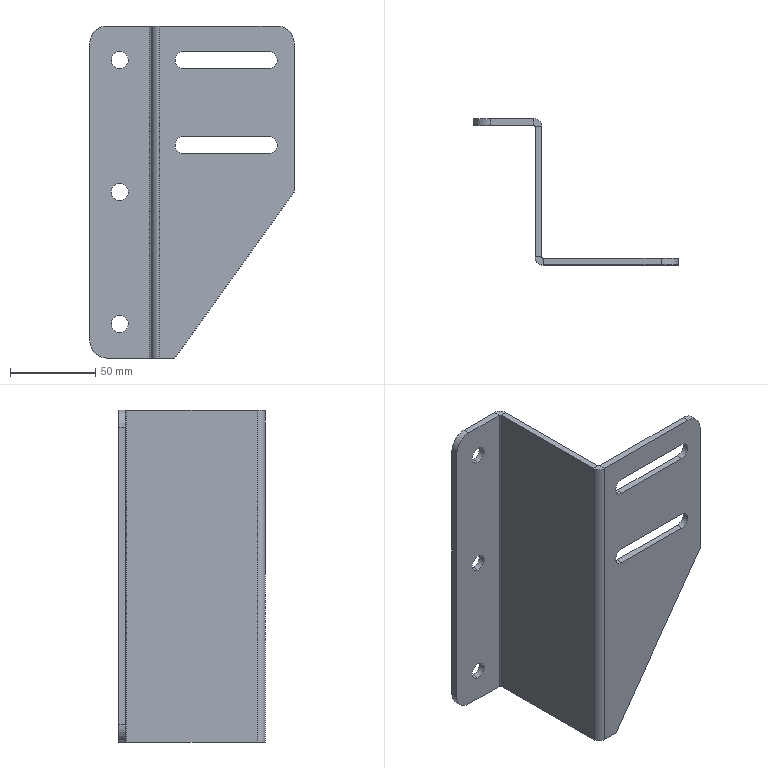Part | SolidWorks | features HoleWzd 2, BreakCorner 1, Cut 1, EdgeFlange 1, ExtruThin 1, FlatPattern 1, SheetMetal 1, SolidToSheetMetal 1 | 1 solid | 40 faces | box 120 x 86 x 195 mm | volume 136249 mm3 | plane 23 | cylinder 17 | commonest cylinder face diameters 10 x10 20 x3 1.473 x2 9.473 x2
STEP:
#1=CARTESIAN_POINT('',(-22.368,78.,-82.5));
#2=VERTEX_POINT('',#1);
#3=CARTESIAN_POINT('',(-22.368,78.,-72.5));
#4=VERTEX_POINT('',#3);
#5=CARTESIAN_POINT('',(-22.368,78.,-77.5));
#6=DIRECTION('',(0.,1.,0.));
#7=DIRECTION('',(-1.,0.,0.));
#8=AXIS2_PLACEMENT_3D('',#5,#6,#7);
#9=CIRCLE('',#8,5.);
#10=EDGE_CURVE('',#2,#4,#9,.T.);
#11=ORIENTED_EDGE('',*,*,#10,.F.);
#12=CARTESIAN_POINT('',(-22.368,82.,-82.5));
#13=VERTEX_POINT('',#12);
#14=CARTESIAN_POINT('',(-22.368,82.,-82.5));
#15=DIRECTION('',(0.,1.,0.));
#16=VECTOR('',#15,1000.);
#17=LINE('',#14,#16);
#18=EDGE_CURVE('',#2,#13,#17,.T.);
#19=ORIENTED_EDGE('',*,*,#18,.T.);
#20=CARTESIAN_POINT('',(-22.368,82.,-72.5));
#21=VERTEX_POINT('',#20);
#22=CARTESIAN_POINT('',(-22.368,82.,-77.5));
#23=DIRECTION('',(0.,1.,0.));
#24=DIRECTION('',(0.,0.,1.));
#25=AXIS2_PLACEMENT_3D('',#22,#23,#24);
#26=CIRCLE('',#25,5.);
#27=EDGE_CURVE('',#13,#21,#26,.T.);
#28=ORIENTED_EDGE('',*,*,#27,.T.);
#29=CARTESIAN_POINT('',(-22.368,82.,-72.5));
#30=DIRECTION('',(0.,1.,0.));
#31=VECTOR('',#30,1000.);
#32=LINE('',#29,#31);
#33=EDGE_CURVE('',#4,#21,#32,.T.);
#34=ORIENTED_EDGE('',*,*,#33,.F.);
#35=EDGE_LOOP('',(#11,#19,#28,#34));
#36=FACE_OUTER_BOUND('',#35,.T.);
#37=CARTESIAN_POINT('',(-22.368,82.,-77.5));
#38=DIRECTION('',(0.,1.,0.));
#39=DIRECTION('',(0.,0.,1.));
#40=AXIS2_PLACEMENT_3D('',#37,#38,#39);
#41=CYLINDRICAL_SURFACE('',#40,5.);
#42=ADVANCED_FACE('',(#36),#41,.F.);
#43=CARTESIAN_POINT('',(-22.368,78.,-5.));
#44=VERTEX_POINT('',#43);
#45=CARTESIAN_POINT('',(-22.368,78.,5.));
#46=VERTEX_POINT('',#45);
#47=CARTESIAN_POINT('',(-22.368,78.,0.));
#48=DIRECTION('',(0.,1.,0.));
#49=DIRECTION('',(-1.,0.,0.));
#50=AXIS2_PLACEMENT_3D('',#47,#48,#49);
#51=CIRCLE('',#50,5.);
#52=EDGE_CURVE('',#44,#46,#51,.T.);
#53=ORIENTED_EDGE('',*,*,#52,.F.);
#54=CARTESIAN_POINT('',(-22.368,82.,-5.));
#55=VERTEX_POINT('',#54);
#56=CARTESIAN_POINT('',(-22.368,82.,-5.));
#57=DIRECTION('',(0.,1.,0.));
#58=VECTOR('',#57,1000.);
#59=LINE('',#56,#58);
#60=EDGE_CURVE('',#44,#55,#59,.T.);
#61=ORIENTED_EDGE('',*,*,#60,.T.);
#62=CARTESIAN_POINT('',(-22.368,82.,5.));
#63=VERTEX_POINT('',#62);
#64=CARTESIAN_POINT('',(-22.368,82.,0.));
#65=DIRECTION('',(0.,1.,0.));
#66=DIRECTION('',(0.,0.,1.));
#67=AXIS2_PLACEMENT_3D('',#64,#65,#66);
#68=CIRCLE('',#67,5.);
#69=EDGE_CURVE('',#55,#63,#68,.T.);
#70=ORIENTED_EDGE('',*,*,#69,.T.);
#71=CARTESIAN_POINT('',(-22.368,82.,5.));
#72=DIRECTION('',(0.,1.,0.));
#73=VECTOR('',#72,1000.);
#74=LINE('',#71,#73);
#75=EDGE_CURVE('',#46,#63,#74,.T.);
#76=ORIENTED_EDGE('',*,*,#75,.F.);
#77=EDGE_LOOP('',(#53,#61,#70,#76));
#78=FACE_OUTER_BOUND('',#77,.T.);
#79=CARTESIAN_POINT('',(-22.368,82.,0.));
#80=DIRECTION('',(0.,1.,0.));
#81=DIRECTION('',(0.,0.,1.));
#82=AXIS2_PLACEMENT_3D('',#79,#80,#81);
#83=CYLINDRICAL_SURFACE('',#82,5.);
#84=ADVANCED_FACE('',(#78),#83,.F.);
#85=CARTESIAN_POINT('',(-22.368,78.,72.5));
#86=VERTEX_POINT('',#85);
#87=CARTESIAN_POINT('',(-22.368,78.,82.5));
#88=VERTEX_POINT('',#87);
#89=CARTESIAN_POINT('',(-22.368,78.,77.5));
#90=DIRECTION('',(0.,1.,0.));
#91=DIRECTION('',(-1.,0.,0.));
#92=AXIS2_PLACEMENT_3D('',#89,#90,#91);
#93=CIRCLE('',#92,5.);
#94=EDGE_CURVE('',#86,#88,#93,.T.);
#95=ORIENTED_EDGE('',*,*,#94,.F.);
#96=CARTESIAN_POINT('',(-22.368,82.,72.5));
#97=VERTEX_POINT('',#96);
#98=CARTESIAN_POINT('',(-22.368,82.,72.5));
#99=DIRECTION('',(0.,1.,0.));
#100=VECTOR('',#99,1000.);
#101=LINE('',#98,#100);
#102=EDGE_CURVE('',#86,#97,#101,.T.);
#103=ORIENTED_EDGE('',*,*,#102,.T.);
#104=CARTESIAN_POINT('',(-22.368,82.,82.5));
#105=VERTEX_POINT('',#104);
#106=CARTESIAN_POINT('',(-22.368,82.,77.5));
#107=DIRECTION('',(0.,1.,0.));
#108=DIRECTION('',(0.,0.,1.));
#109=AXIS2_PLACEMENT_3D('',#106,#107,#108);
#110=CIRCLE('',#109,5.);
#111=EDGE_CURVE('',#97,#105,#110,.T.);
#112=ORIENTED_EDGE('',*,*,#111,.T.);
#113=CARTESIAN_POINT('',(-22.368,82.,82.5));
#114=DIRECTION('',(0.,1.,0.));
#115=VECTOR('',#114,1000.);
#116=LINE('',#113,#115);
#117=EDGE_CURVE('',#88,#105,#116,.T.);
#118=ORIENTED_EDGE('',*,*,#117,.F.);
#119=EDGE_LOOP('',(#95,#103,#112,#118));
#120=FACE_OUTER_BOUND('',#119,.T.);
#121=CARTESIAN_POINT('',(-22.368,82.,77.5));
#122=DIRECTION('',(0.,1.,0.));
#123=DIRECTION('',(0.,0.,1.));
#124=AXIS2_PLACEMENT_3D('',#121,#122,#123);
#125=CYLINDRICAL_SURFACE('',#124,5.);
#126=ADVANCED_FACE('',(#120),#125,.F.);
#127=CARTESIAN_POINT('',(-4.,77.263,-97.5));
#128=VERTEX_POINT('',#127);
#129=CARTESIAN_POINT('',(-4.,0.7366,-97.5));
#130=VERTEX_POINT('',#129);
#131=CARTESIAN_POINT('',(-4.,0.,-97.5));
#132=DIRECTION('',(0.,-1.,0.));
#133=VECTOR('',#132,1000.);
#134=LINE('',#131,#133);
#135=EDGE_CURVE('',#128,#130,#134,.T.);
#136=ORIENTED_EDGE('',*,*,#135,.F.);
#137=CARTESIAN_POINT('',(0.,77.263,-97.5));
#138=VERTEX_POINT('',#137);
#139=CARTESIAN_POINT('',(-4.,77.263,-97.5));
#140=DIRECTION('',(1.,0.,0.));
#141=VECTOR('',#140,1000.);
#142=LINE('',#139,#141);
#143=EDGE_CURVE('',#128,#138,#142,.T.);
#144=ORIENTED_EDGE('',*,*,#143,.T.);
#145=CARTESIAN_POINT('',(0.,0.7366,-97.5));
#146=VERTEX_POINT('',#145);
#147=CARTESIAN_POINT('',(0.,0.,-97.5));
#148=DIRECTION('',(0.,-1.,0.));
#149=VECTOR('',#148,1000.);
#150=LINE('',#147,#149);
#151=EDGE_CURVE('',#138,#146,#150,.T.);
#152=ORIENTED_EDGE('',*,*,#151,.T.);
#153=CARTESIAN_POINT('',(-4.,0.7366,-97.5));
#154=DIRECTION('',(-1.,0.,0.));
#155=VECTOR('',#154,1000.);
#156=LINE('',#153,#155);
#157=EDGE_CURVE('',#146,#130,#156,.T.);
#158=ORIENTED_EDGE('',*,*,#157,.T.);
#159=EDGE_LOOP('',(#136,#144,#152,#158));
#160=FACE_OUTER_BOUND('',#159,.T.);
#161=CARTESIAN_POINT('',(-4.,0.,-97.5));
#162=DIRECTION('',(0.,0.,-1.));
#163=DIRECTION('',(0.,1.,0.));
#164=AXIS2_PLACEMENT_3D('',#161,#162,#163);
#165=PLANE('',#164);
#166=ADVANCED_FACE('',(#160),#165,.T.);
#167=CARTESIAN_POINT('',(-4.,77.263,97.5));
#168=VERTEX_POINT('',#167);
#169=CARTESIAN_POINT('',(-4.,77.263,-97.5));
#170=DIRECTION('',(0.,0.,1.));
#171=VECTOR('',#170,1000.);
#172=LINE('',#169,#171);
#173=EDGE_CURVE('',#128,#168,#172,.T.);
#174=ORIENTED_EDGE('',*,*,#173,.F.);
#175=ORIENTED_EDGE('',*,*,#135,.T.);
#176=CARTESIAN_POINT('',(-4.,0.7366,97.5));
#177=VERTEX_POINT('',#176);
#178=CARTESIAN_POINT('',(-4.,0.7366,97.5));
#179=DIRECTION('',(0.,0.,1.));
#180=VECTOR('',#179,1000.);
#181=LINE('',#178,#180);
#182=EDGE_CURVE('',#130,#177,#181,.T.);
#183=ORIENTED_EDGE('',*,*,#182,.T.);
#184=CARTESIAN_POINT('',(-4.,0.,97.5));
#185=DIRECTION('',(0.,-1.,0.));
#186=VECTOR('',#185,1000.);
#187=LINE('',#184,#186);
#188=EDGE_CURVE('',#168,#177,#187,.T.);
#189=ORIENTED_EDGE('',*,*,#188,.F.);
#190=EDGE_LOOP('',(#174,#175,#183,#189));
#191=FACE_OUTER_BOUND('',#190,.T.);
#192=CARTESIAN_POINT('',(-4.,0.,97.5));
#193=DIRECTION('',(1.,0.,0.));
#194=DIRECTION('',(0.,0.,-1.));
#195=AXIS2_PLACEMENT_3D('',#192,#193,#194);
#196=PLANE('',#195);
#197=ADVANCED_FACE('',(#191),#196,.F.);
#198=ORIENTED_EDGE('',*,*,#151,.F.);
#199=CARTESIAN_POINT('',(0.,77.263,97.5));
#200=VERTEX_POINT('',#199);
#201=CARTESIAN_POINT('',(0.,77.263,-97.5));
#202=DIRECTION('',(0.,0.,1.));
#203=VECTOR('',#202,1000.);
#204=LINE('',#201,#203);
#205=EDGE_CURVE('',#138,#200,#204,.T.);
#206=ORIENTED_EDGE('',*,*,#205,.T.);
#207=CARTESIAN_POINT('',(0.,0.7366,97.5));
#208=VERTEX_POINT('',#207);
#209=CARTESIAN_POINT('',(0.,0.,97.5));
#210=DIRECTION('',(0.,-1.,0.));
#211=VECTOR('',#210,1000.);
#212=LINE('',#209,#211);
#213=EDGE_CURVE('',#200,#208,#212,.T.);
#214=ORIENTED_EDGE('',*,*,#213,.T.);
#215=CARTESIAN_POINT('',(0.,0.7366,97.5));
#216=DIRECTION('',(0.,0.,1.));
#217=VECTOR('',#216,1000.);
#218=LINE('',#215,#217);
#219=EDGE_CURVE('',#146,#208,#218,.T.);
#220=ORIENTED_EDGE('',*,*,#219,.F.);
#221=EDGE_LOOP('',(#198,#206,#214,#220));
#222=FACE_OUTER_BOUND('',#221,.T.);
#223=CARTESIAN_POINT('',(0.,0.,97.5));
#224=DIRECTION('',(1.,0.,0.));
#225=DIRECTION('',(0.,0.,-1.));
#226=AXIS2_PLACEMENT_3D('',#223,#224,#225);
#227=PLANE('',#226);
#228=ADVANCED_FACE('',(#222),#227,.T.);
#229=CARTESIAN_POINT('',(15.,0.,32.5));
#230=VERTEX_POINT('',#229);
#231=CARTESIAN_POINT('',(15.,-4.,32.5));
#232=VERTEX_POINT('',#231);
#233=CARTESIAN_POINT('',(15.,-4.,32.5));
#234=DIRECTION('',(0.,-1.,0.));
#235=VECTOR('',#234,1000.);
#236=LINE('',#233,#235);
#237=EDGE_CURVE('',#230,#232,#236,.T.);
#238=ORIENTED_EDGE('',*,*,#237,.F.);
#239=CARTESIAN_POINT('',(65.,0.,32.5));
#240=VERTEX_POINT('',#239);
#241=CARTESIAN_POINT('',(0.,0.,32.5));
#242=DIRECTION('',(1.,0.,0.));
#243=VECTOR('',#242,1000.);
#244=LINE('',#241,#243);
#245=EDGE_CURVE('',#230,#240,#244,.T.);
#246=ORIENTED_EDGE('',*,*,#245,.T.);
#247=CARTESIAN_POINT('',(65.,-4.,32.5));
#248=VERTEX_POINT('',#247);
#249=CARTESIAN_POINT('',(65.,-4.,32.5));
#250=DIRECTION('',(0.,-1.,0.));
#251=VECTOR('',#250,1000.);
#252=LINE('',#249,#251);
#253=EDGE_CURVE('',#240,#248,#252,.T.);
#254=ORIENTED_EDGE('',*,*,#253,.T.);
#255=CARTESIAN_POINT('',(15.,-4.,32.5));
#256=DIRECTION('',(1.,0.,0.));
#257=VECTOR('',#256,1000.);
#258=LINE('',#255,#257);
#259=EDGE_CURVE('',#232,#248,#258,.T.);
#260=ORIENTED_EDGE('',*,*,#259,.F.);
#261=EDGE_LOOP('',(#238,#246,#254,#260));
#262=FACE_OUTER_BOUND('',#261,.T.);
#263=CARTESIAN_POINT('',(15.,-4.,32.5));
#264=DIRECTION('',(0.,0.,1.));
#265=DIRECTION('',(1.,0.,0.));
#266=AXIS2_PLACEMENT_3D('',#263,#264,#265);
#267=PLANE('',#266);
#268=ADVANCED_FACE('',(#262),#267,.F.);
#269=ORIENTED_EDGE('',*,*,#253,.F.);
#270=CARTESIAN_POINT('',(65.,0.,22.5));
#271=VERTEX_POINT('',#270);
#272=CARTESIAN_POINT('',(65.,0.,27.5));
#273=DIRECTION('',(0.,1.,0.));
#274=DIRECTION('',(0.,0.,1.));
#275=AXIS2_PLACEMENT_3D('',#272,#273,#274);
#276=CIRCLE('',#275,5.);
#277=EDGE_CURVE('',#240,#271,#276,.T.);
#278=ORIENTED_EDGE('',*,*,#277,.T.);
#279=CARTESIAN_POINT('',(65.,-4.,22.5));
#280=VERTEX_POINT('',#279);
#281=CARTESIAN_POINT('',(65.,-4.,22.5));
#282=DIRECTION('',(0.,-1.,0.));
#283=VECTOR('',#282,1000.);
#284=LINE('',#281,#283);
#285=EDGE_CURVE('',#271,#280,#284,.T.);
#286=ORIENTED_EDGE('',*,*,#285,.T.);
#287=CARTESIAN_POINT('',(65.,-4.,27.5));
#288=DIRECTION('',(0.,1.,0.));
#289=DIRECTION('',(0.,0.,1.));
#290=AXIS2_PLACEMENT_3D('',#287,#288,#289);
#291=CIRCLE('',#290,5.);
#292=EDGE_CURVE('',#248,#280,#291,.T.);
#293=ORIENTED_EDGE('',*,*,#292,.F.);
#294=EDGE_LOOP('',(#269,#278,#286,#293));
#295=FACE_OUTER_BOUND('',#294,.T.);
#296=CARTESIAN_POINT('',(65.,-4.,27.5));
#297=DIRECTION('',(0.,1.,0.));
#298=DIRECTION('',(0.,0.,1.));
#299=AXIS2_PLACEMENT_3D('',#296,#297,#298);
#300=CYLINDRICAL_SURFACE('',#299,5.);
#301=ADVANCED_FACE('',(#295),#300,.F.);
#302=ORIENTED_EDGE('',*,*,#285,.F.);
#303=CARTESIAN_POINT('',(15.,0.,22.5));
#304=VERTEX_POINT('',#303);
#305=CARTESIAN_POINT('',(0.,0.,22.5));
#306=DIRECTION('',(1.,0.,0.));
#307=VECTOR('',#306,1000.);
#308=LINE('',#305,#307);
#309=EDGE_CURVE('',#304,#271,#308,.T.);
#310=ORIENTED_EDGE('',*,*,#309,.F.);
#311=CARTESIAN_POINT('',(15.,-4.,22.5));
#312=VERTEX_POINT('',#311);
#313=CARTESIAN_POINT('',(15.,-4.,22.5));
#314=DIRECTION('',(0.,-1.,0.));
#315=VECTOR('',#314,1000.);
#316=LINE('',#313,#315);
#317=EDGE_CURVE('',#304,#312,#316,.T.);
#318=ORIENTED_EDGE('',*,*,#317,.T.);
#319=CARTESIAN_POINT('',(15.,-4.,22.5));
#320=DIRECTION('',(1.,0.,0.));
#321=VECTOR('',#320,1000.);
#322=LINE('',#319,#321);
#323=EDGE_CURVE('',#312,#280,#322,.T.);
#324=ORIENTED_EDGE('',*,*,#323,.T.);
#325=EDGE_LOOP('',(#302,#310,#318,#324));
#326=FACE_OUTER_BOUND('',#325,.T.);
#327=CARTESIAN_POINT('',(15.,-4.,22.5));
#328=DIRECTION('',(0.,0.,1.));
#329=DIRECTION('',(1.,0.,0.));
#330=AXIS2_PLACEMENT_3D('',#327,#328,#329);
#331=PLANE('',#330);
#332=ADVANCED_FACE('',(#326),#331,.T.);
#333=CARTESIAN_POINT('',(15.,0.,82.5));
#334=VERTEX_POINT('',#333);
#335=CARTESIAN_POINT('',(15.,-4.,82.5));
#336=VERTEX_POINT('',#335);
#337=CARTESIAN_POINT('',(15.,-4.,82.5));
#338=DIRECTION('',(0.,-1.,0.));
#339=VECTOR('',#338,1000.);
#340=LINE('',#337,#339);
#341=EDGE_CURVE('',#334,#336,#340,.T.);
#342=ORIENTED_EDGE('',*,*,#341,.F.);
#343=CARTESIAN_POINT('',(65.,0.,82.5));
#344=VERTEX_POINT('',#343);
#345=CARTESIAN_POINT('',(0.,0.,82.5));
#346=DIRECTION('',(1.,0.,0.));
#347=VECTOR('',#346,1000.);
#348=LINE('',#345,#347);
#349=EDGE_CURVE('',#334,#344,#348,.T.);
#350=ORIENTED_EDGE('',*,*,#349,.T.);
#351=CARTESIAN_POINT('',(65.,-4.,82.5));
#352=VERTEX_POINT('',#351);
#353=CARTESIAN_POINT('',(65.,-4.,82.5));
#354=DIRECTION('',(0.,-1.,0.));
#355=VECTOR('',#354,1000.);
#356=LINE('',#353,#355);
#357=EDGE_CURVE('',#344,#352,#356,.T.);
#358=ORIENTED_EDGE('',*,*,#357,.T.);
#359=CARTESIAN_POINT('',(15.,-4.,82.5));
#360=DIRECTION('',(1.,0.,0.));
#361=VECTOR('',#360,1000.);
#362=LINE('',#359,#361);
#363=EDGE_CURVE('',#336,#352,#362,.T.);
#364=ORIENTED_EDGE('',*,*,#363,.F.);
#365=EDGE_LOOP('',(#342,#350,#358,#364));
#366=FACE_OUTER_BOUND('',#365,.T.);
#367=CARTESIAN_POINT('',(15.,-4.,82.5));
#368=DIRECTION('',(0.,0.,1.));
#369=DIRECTION('',(1.,0.,0.));
#370=AXIS2_PLACEMENT_3D('',#367,#368,#369);
#371=PLANE('',#370);
#372=ADVANCED_FACE('',(#366),#371,.F.);
#373=ORIENTED_EDGE('',*,*,#357,.F.);
#374=CARTESIAN_POINT('',(65.,0.,72.5));
#375=VERTEX_POINT('',#374);
#376=CARTESIAN_POINT('',(65.,0.,77.5));
#377=DIRECTION('',(0.,1.,0.));
#378=DIRECTION('',(0.,0.,1.));
#379=AXIS2_PLACEMENT_3D('',#376,#377,#378);
#380=CIRCLE('',#379,5.);
#381=EDGE_CURVE('',#344,#375,#380,.T.);
#382=ORIENTED_EDGE('',*,*,#381,.T.);
#383=CARTESIAN_POINT('',(65.,-4.,72.5));
#384=VERTEX_POINT('',#383);
#385=CARTESIAN_POINT('',(65.,-4.,72.5));
#386=DIRECTION('',(0.,-1.,0.));
#387=VECTOR('',#386,1000.);
#388=LINE('',#385,#387);
#389=EDGE_CURVE('',#375,#384,#388,.T.);
#390=ORIENTED_EDGE('',*,*,#389,.T.);
#391=CARTESIAN_POINT('',(65.,-4.,77.5));
#392=DIRECTION('',(0.,1.,0.));
#393=DIRECTION('',(0.,0.,1.));
#394=AXIS2_PLACEMENT_3D('',#391,#392,#393);
#395=CIRCLE('',#394,5.);
#396=EDGE_CURVE('',#352,#384,#395,.T.);
#397=ORIENTED_EDGE('',*,*,#396,.F.);
#398=EDGE_LOOP('',(#373,#382,#390,#397));
#399=FACE_OUTER_BOUND('',#398,.T.);
#400=CARTESIAN_POINT('',(65.,-4.,77.5));
#401=DIRECTION('',(0.,1.,0.));
#402=DIRECTION('',(0.,0.,1.));
#403=AXIS2_PLACEMENT_3D('',#400,#401,#402);
#404=CYLINDRICAL_SURFACE('',#403,5.);
#405=ADVANCED_FACE('',(#399),#404,.F.);
#406=ORIENTED_EDGE('',*,*,#389,.F.);
#407=CARTESIAN_POINT('',(15.,0.,72.5));
#408=VERTEX_POINT('',#407);
#409=CARTESIAN_POINT('',(0.,0.,72.5));
#410=DIRECTION('',(1.,0.,0.));
#411=VECTOR('',#410,1000.);
#412=LINE('',#409,#411);
#413=EDGE_CURVE('',#408,#375,#412,.T.);
#414=ORIENTED_EDGE('',*,*,#413,.F.);
#415=CARTESIAN_POINT('',(15.,-4.,72.5));
#416=VERTEX_POINT('',#415);
#417=CARTESIAN_POINT('',(15.,-4.,72.5));
#418=DIRECTION('',(0.,-1.,0.));
#419=VECTOR('',#418,1000.);
#420=LINE('',#417,#419);
#421=EDGE_CURVE('',#408,#416,#420,.T.);
#422=ORIENTED_EDGE('',*,*,#421,.T.);
#423=CARTESIAN_POINT('',(15.,-4.,72.5));
#424=DIRECTION('',(1.,0.,0.));
#425=VECTOR('',#424,1000.);
#426=LINE('',#423,#425);
#427=EDGE_CURVE('',#416,#384,#426,.T.);
#428=ORIENTED_EDGE('',*,*,#427,.T.);
#429=EDGE_LOOP('',(#406,#414,#422,#428));
#430=FACE_OUTER_BOUND('',#429,.T.);
#431=CARTESIAN_POINT('',(15.,-4.,72.5));
#432=DIRECTION('',(0.,0.,1.));
#433=DIRECTION('',(1.,0.,0.));
#434=AXIS2_PLACEMENT_3D('',#431,#432,#433);
#435=PLANE('',#434);
#436=ADVANCED_FACE('',(#430),#435,.T.);
#437=CARTESIAN_POINT('',(10.,-4.,-97.5));
#438=VERTEX_POINT('',#437);
#439=CARTESIAN_POINT('',(10.,0.,-97.5));
#440=VERTEX_POINT('',#439);
#441=CARTESIAN_POINT('',(10.,-4.,-97.5));
#442=DIRECTION('',(0.,1.,0.));
#443=VECTOR('',#442,1000.);
#444=LINE('',#441,#443);
#445=EDGE_CURVE('',#438,#440,#444,.T.);
#446=ORIENTED_EDGE('',*,*,#445,.F.);
#447=CARTESIAN_POINT('',(0.7366,-4.,-97.5));
#448=VERTEX_POINT('',#447);
#449=CARTESIAN_POINT('',(0.,-4.,-97.5));
#450=DIRECTION('',(1.,0.,0.));
#451=VECTOR('',#450,1000.);
#452=LINE('',#449,#451);
#453=EDGE_CURVE('',#448,#438,#452,.T.);
#454=ORIENTED_EDGE('',*,*,#453,.F.);
#455=CARTESIAN_POINT('',(0.7366,0.,-97.5));
#456=VERTEX_POINT('',#455);
#457=CARTESIAN_POINT('',(0.7366,-4.,-97.5));
#458=DIRECTION('',(0.,-1.,0.));
#459=VECTOR('',#458,1000.);
#460=LINE('',#457,#459);
#461=EDGE_CURVE('',#456,#448,#460,.T.);
#462=ORIENTED_EDGE('',*,*,#461,.F.);
#463=CARTESIAN_POINT('',(0.,0.,-97.5));
#464=DIRECTION('',(1.,0.,0.));
#465=VECTOR('',#464,1000.);
#466=LINE('',#463,#465);
#467=EDGE_CURVE('',#456,#440,#466,.T.);
#468=ORIENTED_EDGE('',*,*,#467,.T.);
#469=EDGE_LOOP('',(#446,#454,#462,#468));
#470=FACE_OUTER_BOUND('',#469,.T.);
#471=CARTESIAN_POINT('',(0.,-4.,-97.5));
#472=DIRECTION('',(0.,0.,1.));
#473=DIRECTION('',(1.,0.,0.));
#474=AXIS2_PLACEMENT_3D('',#471,#472,#473);
#475=PLANE('',#474);
#476=ADVANCED_FACE('',(#470),#475,.F.);
#477=CARTESIAN_POINT('',(80.,0.,87.5));
#478=VERTEX_POINT('',#477);
#479=CARTESIAN_POINT('',(80.,0.,0.));
#480=VERTEX_POINT('',#479);
#481=CARTESIAN_POINT('',(80.,0.,97.5));
#482=DIRECTION('',(0.,0.,-1.));
#483=VECTOR('',#482,1000.);
#484=LINE('',#481,#483);
#485=EDGE_CURVE('',#478,#480,#484,.T.);
#486=ORIENTED_EDGE('',*,*,#485,.F.);
#487=CARTESIAN_POINT('',(80.,-4.,87.5));
#488=VERTEX_POINT('',#487);
#489=CARTESIAN_POINT('',(80.,-4.,87.5));
#490=DIRECTION('',(0.,-1.,0.));
#491=VECTOR('',#490,1000.);
#492=LINE('',#489,#491);
#493=EDGE_CURVE('',#478,#488,#492,.T.);
#494=ORIENTED_EDGE('',*,*,#493,.T.);
#495=CARTESIAN_POINT('',(80.,-4.,0.));
#496=VERTEX_POINT('',#495);
#497=CARTESIAN_POINT('',(80.,-4.,97.5));
#498=DIRECTION('',(0.,0.,-1.));
#499=VECTOR('',#498,1000.);
#500=LINE('',#497,#499);
#501=EDGE_CURVE('',#488,#496,#500,.T.);
#502=ORIENTED_EDGE('',*,*,#501,.T.);
#503=CARTESIAN_POINT('',(80.,-4.,0.));
#504=DIRECTION('',(0.,1.,0.));
#505=VECTOR('',#504,1000.);
#506=LINE('',#503,#505);
#507=EDGE_CURVE('',#496,#480,#506,.T.);
#508=ORIENTED_EDGE('',*,*,#507,.T.);
#509=EDGE_LOOP('',(#486,#494,#502,#508));
#510=FACE_OUTER_BOUND('',#509,.T.);
#511=CARTESIAN_POINT('',(80.,-4.,97.5));
#512=DIRECTION('',(1.,0.,0.));
#513=DIRECTION('',(0.,0.,-1.));
#514=AXIS2_PLACEMENT_3D('',#511,#512,#513);
#515=PLANE('',#514);
#516=ADVANCED_FACE('',(#510),#515,.T.);
#517=CARTESIAN_POINT('',(0.7366,-4.,97.5));
#518=VERTEX_POINT('',#517);
#519=CARTESIAN_POINT('',(70.,-4.,97.5));
#520=VERTEX_POINT('',#519);
#521=CARTESIAN_POINT('',(0.,-4.,97.5));
#522=DIRECTION('',(1.,0.,0.));
#523=VECTOR('',#522,1000.);
#524=LINE('',#521,#523);
#525=EDGE_CURVE('',#518,#520,#524,.T.);
#526=ORIENTED_EDGE('',*,*,#525,.T.);
#527=CARTESIAN_POINT('',(70.,0.,97.5));
#528=VERTEX_POINT('',#527);
#529=CARTESIAN_POINT('',(70.,-4.,97.5));
#530=DIRECTION('',(0.,1.,0.));
#531=VECTOR('',#530,1000.);
#532=LINE('',#529,#531);
#533=EDGE_CURVE('',#520,#528,#532,.T.);
#534=ORIENTED_EDGE('',*,*,#533,.T.);
#535=CARTESIAN_POINT('',(0.7366,0.,97.5));
#536=VERTEX_POINT('',#535);
#537=CARTESIAN_POINT('',(0.,0.,97.5));
#538=DIRECTION('',(1.,0.,0.));
#539=VECTOR('',#538,1000.);
#540=LINE('',#537,#539);
#541=EDGE_CURVE('',#536,#528,#540,.T.);
#542=ORIENTED_EDGE('',*,*,#541,.F.);
#543=CARTESIAN_POINT('',(0.7366,-4.,97.5));
#544=DIRECTION('',(0.,-1.,0.));
#545=VECTOR('',#544,1000.);
#546=LINE('',#543,#545);
#547=EDGE_CURVE('',#536,#518,#546,.T.);
#548=ORIENTED_EDGE('',*,*,#547,.T.);
#549=EDGE_LOOP('',(#526,#534,#542,#548));
#550=FACE_OUTER_BOUND('',#549,.T.);
#551=CARTESIAN_POINT('',(0.,-4.,97.5));
#552=DIRECTION('',(0.,0.,1.));
#553=DIRECTION('',(1.,0.,0.));
#554=AXIS2_PLACEMENT_3D('',#551,#552,#553);
#555=PLANE('',#554);
#556=ADVANCED_FACE('',(#550),#555,.T.);
#557=ORIENTED_EDGE('',*,*,#547,.F.);
#558=CARTESIAN_POINT('',(0.7366,0.7366,97.5));
#559=DIRECTION('',(0.,0.,-1.));
#560=DIRECTION('',(-1.,0.,0.));
#561=AXIS2_PLACEMENT_3D('',#558,#559,#560);
#562=CIRCLE('',#561,0.7366);
#563=EDGE_CURVE('',#536,#208,#562,.T.);
#564=ORIENTED_EDGE('',*,*,#563,.T.);
#565=CARTESIAN_POINT('',(-4.,0.7366,97.5));
#566=DIRECTION('',(-1.,0.,0.));
#567=VECTOR('',#566,1000.);
#568=LINE('',#565,#567);
#569=EDGE_CURVE('',#208,#177,#568,.T.);
#570=ORIENTED_EDGE('',*,*,#569,.T.);
#571=CARTESIAN_POINT('',(0.7366,0.7366,97.5));
#572=DIRECTION('',(0.,0.,-1.));
#573=DIRECTION('',(-1.,0.,0.));
#574=AXIS2_PLACEMENT_3D('',#571,#572,#573);
#575=CIRCLE('',#574,4.737);
#576=EDGE_CURVE('',#518,#177,#575,.T.);
#577=ORIENTED_EDGE('',*,*,#576,.F.);
#578=EDGE_LOOP('',(#557,#564,#570,#577));
#579=FACE_OUTER_BOUND('',#578,.T.);
#580=CARTESIAN_POINT('',(0.7366,0.7366,97.5));
#581=DIRECTION('',(0.,0.,1.));
#582=DIRECTION('',(1.,0.,0.));
#583=AXIS2_PLACEMENT_3D('',#580,#581,#582);
#584=PLANE('',#583);
#585=ADVANCED_FACE('',(#579),#584,.T.);
#586=CARTESIAN_POINT('',(-4.,77.263,97.5));
#587=DIRECTION('',(1.,0.,0.));
#588=VECTOR('',#587,1000.);
#589=LINE('',#586,#588);
#590=EDGE_CURVE('',#168,#200,#589,.T.);
#591=ORIENTED_EDGE('',*,*,#590,.F.);
#592=ORIENTED_EDGE('',*,*,#188,.T.);
#593=ORIENTED_EDGE('',*,*,#569,.F.);
#594=ORIENTED_EDGE('',*,*,#213,.F.);
#595=EDGE_LOOP('',(#591,#592,#593,#594));
#596=FACE_OUTER_BOUND('',#595,.T.);
#597=CARTESIAN_POINT('',(-4.,0.,97.5));
#598=DIRECTION('',(0.,0.,-1.));
#599=DIRECTION('',(0.,1.,0.));
#600=AXIS2_PLACEMENT_3D('',#597,#598,#599);
#601=PLANE('',#600);
#602=ADVANCED_FACE('',(#596),#601,.F.);
#603=CARTESIAN_POINT('',(15.,0.,77.5));
#604=DIRECTION('',(0.,1.,0.));
#605=DIRECTION('',(0.,0.,1.));
#606=AXIS2_PLACEMENT_3D('',#603,#604,#605);
#607=CIRCLE('',#606,5.);
#608=EDGE_CURVE('',#408,#334,#607,.T.);
#609=ORIENTED_EDGE('',*,*,#608,.T.);
#610=ORIENTED_EDGE('',*,*,#341,.T.);
#611=CARTESIAN_POINT('',(15.,-4.,77.5));
#612=DIRECTION('',(0.,1.,0.));
#613=DIRECTION('',(0.,0.,1.));
#614=AXIS2_PLACEMENT_3D('',#611,#612,#613);
#615=CIRCLE('',#614,5.);
#616=EDGE_CURVE('',#416,#336,#615,.T.);
#617=ORIENTED_EDGE('',*,*,#616,.F.);
#618=ORIENTED_EDGE('',*,*,#421,.F.);
#619=EDGE_LOOP('',(#609,#610,#617,#618));
#620=FACE_OUTER_BOUND('',#619,.T.);
#621=CARTESIAN_POINT('',(15.,-4.,77.5));
#622=DIRECTION('',(0.,1.,0.));
#623=DIRECTION('',(0.,0.,1.));
#624=AXIS2_PLACEMENT_3D('',#621,#622,#623);
#625=CYLINDRICAL_SURFACE('',#624,5.);
#626=ADVANCED_FACE('',(#620),#625,.F.);
#627=CARTESIAN_POINT('',(15.,0.,27.5));
#628=DIRECTION('',(0.,1.,0.));
#629=DIRECTION('',(0.,0.,1.));
#630=AXIS2_PLACEMENT_3D('',#627,#628,#629);
#631=CIRCLE('',#630,5.);
#632=EDGE_CURVE('',#304,#230,#631,.T.);
#633=ORIENTED_EDGE('',*,*,#632,.T.);
#634=ORIENTED_EDGE('',*,*,#237,.T.);
#635=CARTESIAN_POINT('',(15.,-4.,27.5));
#636=DIRECTION('',(0.,1.,0.));
#637=DIRECTION('',(0.,0.,1.));
#638=AXIS2_PLACEMENT_3D('',#635,#636,#637);
#639=CIRCLE('',#638,5.);
#640=EDGE_CURVE('',#312,#232,#639,.T.);
#641=ORIENTED_EDGE('',*,*,#640,.F.);
#642=ORIENTED_EDGE('',*,*,#317,.F.);
#643=EDGE_LOOP('',(#633,#634,#641,#642));
#644=FACE_OUTER_BOUND('',#643,.T.);
#645=CARTESIAN_POINT('',(15.,-4.,27.5));
#646=DIRECTION('',(0.,1.,0.));
#647=DIRECTION('',(0.,0.,1.));
#648=AXIS2_PLACEMENT_3D('',#645,#646,#647);
#649=CYLINDRICAL_SURFACE('',#648,5.);
#650=ADVANCED_FACE('',(#644),#649,.F.);
#651=CARTESIAN_POINT('',(0.7366,0.7366,-97.5));
#652=DIRECTION('',(0.,0.,1.));
#653=DIRECTION('',(-1.,0.,0.));
#654=AXIS2_PLACEMENT_3D('',#651,#652,#653);
#655=CIRCLE('',#654,0.7366);
#656=EDGE_CURVE('',#146,#456,#655,.T.);
#657=ORIENTED_EDGE('',*,*,#656,.T.);
#658=ORIENTED_EDGE('',*,*,#461,.T.);
#659=CARTESIAN_POINT('',(0.7366,0.7366,-97.5));
#660=DIRECTION('',(0.,0.,1.));
#661=DIRECTION('',(1.,0.,0.));
#662=AXIS2_PLACEMENT_3D('',#659,#660,#661);
#663=CIRCLE('',#662,4.737);
#664=EDGE_CURVE('',#130,#448,#663,.T.);
#665=ORIENTED_EDGE('',*,*,#664,.F.);
#666=ORIENTED_EDGE('',*,*,#157,.F.);
#667=EDGE_LOOP('',(#657,#658,#665,#666));
#668=FACE_OUTER_BOUND('',#667,.T.);
#669=CARTESIAN_POINT('',(0.7366,0.7366,-97.5));
#670=DIRECTION('',(0.,0.,-1.));
#671=DIRECTION('',(-1.,0.,0.));
#672=AXIS2_PLACEMENT_3D('',#669,#670,#671);
#673=PLANE('',#672);
#674=ADVANCED_FACE('',(#668),#673,.T.);
#675=ORIENTED_EDGE('',*,*,#427,.F.);
#676=ORIENTED_EDGE('',*,*,#616,.T.);
#677=ORIENTED_EDGE('',*,*,#363,.T.);
#678=ORIENTED_EDGE('',*,*,#396,.T.);
#679=EDGE_LOOP('',(#675,#676,#677,#678));
#680=FACE_BOUND('',#679,.T.);
#681=ORIENTED_EDGE('',*,*,#501,.F.);
#682=CARTESIAN_POINT('',(70.,-4.,87.5));
#683=DIRECTION('',(0.,-1.,0.));
#684=DIRECTION('',(0.,0.,1.));
#685=AXIS2_PLACEMENT_3D('',#682,#683,#684);
#686=CIRCLE('',#685,10.);
#687=EDGE_CURVE('',#488,#520,#686,.T.);
#688=ORIENTED_EDGE('',*,*,#687,.T.);
#689=ORIENTED_EDGE('',*,*,#525,.F.);
#690=CARTESIAN_POINT('',(0.7366,-4.,97.5));
#691=DIRECTION('',(0.,0.,-1.));
#692=VECTOR('',#691,1000.);
#693=LINE('',#690,#692);
#694=EDGE_CURVE('',#518,#448,#693,.T.);
#695=ORIENTED_EDGE('',*,*,#694,.T.);
#696=ORIENTED_EDGE('',*,*,#453,.T.);
#697=CARTESIAN_POINT('',(80.,-4.,0.));
#698=DIRECTION('',(0.5832,0.,0.8123));
#699=VECTOR('',#698,1000.);
#700=LINE('',#697,#699);
#701=EDGE_CURVE('',#438,#496,#700,.T.);
#702=ORIENTED_EDGE('',*,*,#701,.T.);
#703=EDGE_LOOP('',(#681,#688,#689,#695,#696,#702));
#704=FACE_OUTER_BOUND('',#703,.T.);
#705=ORIENTED_EDGE('',*,*,#323,.F.);
#706=ORIENTED_EDGE('',*,*,#640,.T.);
#707=ORIENTED_EDGE('',*,*,#259,.T.);
#708=ORIENTED_EDGE('',*,*,#292,.T.);
#709=EDGE_LOOP('',(#705,#706,#707,#708));
#710=FACE_BOUND('',#709,.T.);
#711=CARTESIAN_POINT('',(0.,-4.,97.5));
#712=DIRECTION('',(0.,1.,0.));
#713=DIRECTION('',(0.,0.,1.));
#714=AXIS2_PLACEMENT_3D('',#711,#712,#713);
#715=PLANE('',#714);
#716=ADVANCED_FACE('',(#680,#704,#710),#715,.F.);
#717=ORIENTED_EDGE('',*,*,#576,.T.);
#718=ORIENTED_EDGE('',*,*,#182,.F.);
#719=ORIENTED_EDGE('',*,*,#664,.T.);
#720=ORIENTED_EDGE('',*,*,#694,.F.);
#721=EDGE_LOOP('',(#717,#718,#719,#720));
#722=FACE_OUTER_BOUND('',#721,.T.);
#723=CARTESIAN_POINT('',(0.7366,0.7366,97.5));
#724=DIRECTION('',(0.,0.,-1.));
#725=DIRECTION('',(-1.,0.,0.));
#726=AXIS2_PLACEMENT_3D('',#723,#724,#725);
#727=CYLINDRICAL_SURFACE('',#726,4.737);
#728=ADVANCED_FACE('',(#722),#727,.T.);
#729=ORIENTED_EDGE('',*,*,#541,.T.);
#730=CARTESIAN_POINT('',(70.,0.,87.5));
#731=DIRECTION('',(0.,1.,0.));
#732=DIRECTION('',(0.,0.,1.));
#733=AXIS2_PLACEMENT_3D('',#730,#731,#732);
#734=CIRCLE('',#733,10.);
#735=EDGE_CURVE('',#528,#478,#734,.T.);
#736=ORIENTED_EDGE('',*,*,#735,.T.);
#737=ORIENTED_EDGE('',*,*,#485,.T.);
#738=CARTESIAN_POINT('',(80.,0.,0.));
#739=DIRECTION('',(0.5832,0.,0.8123));
#740=VECTOR('',#739,1000.);
#741=LINE('',#738,#740);
#742=EDGE_CURVE('',#440,#480,#741,.T.);
#743=ORIENTED_EDGE('',*,*,#742,.F.);
#744=ORIENTED_EDGE('',*,*,#467,.F.);
#745=CARTESIAN_POINT('',(0.7366,0.,97.5));
#746=DIRECTION('',(0.,0.,-1.));
#747=VECTOR('',#746,1000.);
#748=LINE('',#745,#747);
#749=EDGE_CURVE('',#536,#456,#748,.T.);
#750=ORIENTED_EDGE('',*,*,#749,.F.);
#751=EDGE_LOOP('',(#729,#736,#737,#743,#744,#750));
#752=FACE_OUTER_BOUND('',#751,.T.);
#753=ORIENTED_EDGE('',*,*,#413,.T.);
#754=ORIENTED_EDGE('',*,*,#381,.F.);
#755=ORIENTED_EDGE('',*,*,#349,.F.);
#756=ORIENTED_EDGE('',*,*,#608,.F.);
#757=EDGE_LOOP('',(#753,#754,#755,#756));
#758=FACE_BOUND('',#757,.T.);
#759=ORIENTED_EDGE('',*,*,#309,.T.);
#760=ORIENTED_EDGE('',*,*,#277,.F.);
#761=ORIENTED_EDGE('',*,*,#245,.F.);
#762=ORIENTED_EDGE('',*,*,#632,.F.);
#763=EDGE_LOOP('',(#759,#760,#761,#762));
#764=FACE_BOUND('',#763,.T.);
#765=CARTESIAN_POINT('',(0.,0.,97.5));
#766=DIRECTION('',(0.,1.,0.));
#767=DIRECTION('',(0.,0.,1.));
#768=AXIS2_PLACEMENT_3D('',#765,#766,#767);
#769=PLANE('',#768);
#770=ADVANCED_FACE('',(#752,#758,#764),#769,.T.);
#771=ORIENTED_EDGE('',*,*,#563,.F.);
#772=ORIENTED_EDGE('',*,*,#749,.T.);
#773=ORIENTED_EDGE('',*,*,#656,.F.);
#774=ORIENTED_EDGE('',*,*,#219,.T.);
#775=EDGE_LOOP('',(#771,#772,#773,#774));
#776=FACE_OUTER_BOUND('',#775,.T.);
#777=CARTESIAN_POINT('',(0.7366,0.7366,97.5));
#778=DIRECTION('',(0.,0.,-1.));
#779=DIRECTION('',(-1.,0.,0.));
#780=AXIS2_PLACEMENT_3D('',#777,#778,#779);
#781=CYLINDRICAL_SURFACE('',#780,0.7366);
#782=ADVANCED_FACE('',(#776),#781,.F.);
#783=CARTESIAN_POINT('',(-4.737,78.,97.5));
#784=VERTEX_POINT('',#783);
#785=CARTESIAN_POINT('',(-4.737,82.,97.5));
#786=VERTEX_POINT('',#785);
#787=CARTESIAN_POINT('',(-4.737,82.,97.5));
#788=DIRECTION('',(0.,1.,0.));
#789=VECTOR('',#788,1000.);
#790=LINE('',#787,#789);
#791=EDGE_CURVE('',#784,#786,#790,.T.);
#792=ORIENTED_EDGE('',*,*,#791,.F.);
#793=CARTESIAN_POINT('',(-4.737,77.263,97.5));
#794=DIRECTION('',(0.,0.,1.));
#795=DIRECTION('',(-1.,0.,0.));
#796=AXIS2_PLACEMENT_3D('',#793,#794,#795);
#797=CIRCLE('',#796,0.7366);
#798=EDGE_CURVE('',#168,#784,#797,.T.);
#799=ORIENTED_EDGE('',*,*,#798,.F.);
#800=ORIENTED_EDGE('',*,*,#590,.T.);
#801=CARTESIAN_POINT('',(-4.737,77.263,97.5));
#802=DIRECTION('',(0.,0.,1.));
#803=DIRECTION('',(-1.,0.,0.));
#804=AXIS2_PLACEMENT_3D('',#801,#802,#803);
#805=CIRCLE('',#804,4.737);
#806=EDGE_CURVE('',#200,#786,#805,.T.);
#807=ORIENTED_EDGE('',*,*,#806,.T.);
#808=EDGE_LOOP('',(#792,#799,#800,#807));
#809=FACE_OUTER_BOUND('',#808,.T.);
#810=CARTESIAN_POINT('',(-4.737,77.263,97.5));
#811=DIRECTION('',(0.,0.,1.));
#812=DIRECTION('',(1.,0.,0.));
#813=AXIS2_PLACEMENT_3D('',#810,#811,#812);
#814=PLANE('',#813);
#815=ADVANCED_FACE('',(#809),#814,.T.);
#816=CARTESIAN_POINT('',(-4.737,78.,-97.5));
#817=VERTEX_POINT('',#816);
#818=CARTESIAN_POINT('',(-4.737,77.263,-97.5));
#819=DIRECTION('',(0.,0.,-1.));
#820=DIRECTION('',(-1.,0.,0.));
#821=AXIS2_PLACEMENT_3D('',#818,#819,#820);
#822=CIRCLE('',#821,0.7366);
#823=EDGE_CURVE('',#817,#128,#822,.T.);
#824=ORIENTED_EDGE('',*,*,#823,.F.);
#825=CARTESIAN_POINT('',(-4.737,82.,-97.5));
#826=VERTEX_POINT('',#825);
#827=CARTESIAN_POINT('',(-4.737,78.,-97.5));
#828=DIRECTION('',(0.,1.,0.));
#829=VECTOR('',#828,1000.);
#830=LINE('',#827,#829);
#831=EDGE_CURVE('',#817,#826,#830,.T.);
#832=ORIENTED_EDGE('',*,*,#831,.T.);
#833=CARTESIAN_POINT('',(-4.737,77.263,-97.5));
#834=DIRECTION('',(0.,0.,-1.));
#835=DIRECTION('',(-1.,0.,0.));
#836=AXIS2_PLACEMENT_3D('',#833,#834,#835);
#837=CIRCLE('',#836,4.737);
#838=EDGE_CURVE('',#826,#138,#837,.T.);
#839=ORIENTED_EDGE('',*,*,#838,.T.);
#840=ORIENTED_EDGE('',*,*,#143,.F.);
#841=EDGE_LOOP('',(#824,#832,#839,#840));
#842=FACE_OUTER_BOUND('',#841,.T.);
#843=CARTESIAN_POINT('',(-4.737,77.263,-97.5));
#844=DIRECTION('',(0.,0.,1.));
#845=DIRECTION('',(1.,0.,0.));
#846=AXIS2_PLACEMENT_3D('',#843,#844,#845);
#847=PLANE('',#846);
#848=ADVANCED_FACE('',(#842),#847,.F.);
#849=ORIENTED_EDGE('',*,*,#205,.F.);
#850=ORIENTED_EDGE('',*,*,#838,.F.);
#851=CARTESIAN_POINT('',(-4.737,82.,0.));
#852=DIRECTION('',(0.,0.,-1.));
#853=VECTOR('',#852,1000.);
#854=LINE('',#851,#853);
#855=EDGE_CURVE('',#786,#826,#854,.T.);
#856=ORIENTED_EDGE('',*,*,#855,.F.);
#857=ORIENTED_EDGE('',*,*,#806,.F.);
#858=EDGE_LOOP('',(#849,#850,#856,#857));
#859=FACE_OUTER_BOUND('',#858,.T.);
#860=CARTESIAN_POINT('',(-4.737,77.263,-97.5));
#861=DIRECTION('',(0.,0.,-1.));
#862=DIRECTION('',(0.,1.,0.));
#863=AXIS2_PLACEMENT_3D('',#860,#861,#862);
#864=CYLINDRICAL_SURFACE('',#863,4.737);
#865=ADVANCED_FACE('',(#859),#864,.T.);
#866=ORIENTED_EDGE('',*,*,#173,.T.);
#867=ORIENTED_EDGE('',*,*,#798,.T.);
#868=CARTESIAN_POINT('',(-4.737,78.,97.5));
#869=DIRECTION('',(0.,0.,-1.));
#870=VECTOR('',#869,1000.);
#871=LINE('',#868,#870);
#872=EDGE_CURVE('',#784,#817,#871,.T.);
#873=ORIENTED_EDGE('',*,*,#872,.T.);
#874=ORIENTED_EDGE('',*,*,#823,.T.);
#875=EDGE_LOOP('',(#866,#867,#873,#874));
#876=FACE_OUTER_BOUND('',#875,.T.);
#877=CARTESIAN_POINT('',(-4.737,77.263,-97.5));
#878=DIRECTION('',(0.,0.,-1.));
#879=DIRECTION('',(0.,1.,0.));
#880=AXIS2_PLACEMENT_3D('',#877,#878,#879);
#881=CYLINDRICAL_SURFACE('',#880,0.7366);
#882=ADVANCED_FACE('',(#876),#881,.F.);
#883=CARTESIAN_POINT('',(-30.,78.,-97.5));
#884=VERTEX_POINT('',#883);
#885=CARTESIAN_POINT('',(0.,78.,-97.5));
#886=DIRECTION('',(1.,0.,0.));
#887=VECTOR('',#886,1000.);
#888=LINE('',#885,#887);
#889=EDGE_CURVE('',#884,#817,#888,.T.);
#890=ORIENTED_EDGE('',*,*,#889,.F.);
#891=CARTESIAN_POINT('',(-30.,82.,-97.5));
#892=VERTEX_POINT('',#891);
#893=CARTESIAN_POINT('',(-30.,82.,-97.5));
#894=DIRECTION('',(0.,1.,0.));
#895=VECTOR('',#894,1000.);
#896=LINE('',#893,#895);
#897=EDGE_CURVE('',#884,#892,#896,.T.);
#898=ORIENTED_EDGE('',*,*,#897,.T.);
#899=CARTESIAN_POINT('',(-4.,82.,-97.5));
#900=DIRECTION('',(1.,0.,0.));
#901=VECTOR('',#900,1000.);
#902=LINE('',#899,#901);
#903=EDGE_CURVE('',#892,#826,#902,.T.);
#904=ORIENTED_EDGE('',*,*,#903,.T.);
#905=ORIENTED_EDGE('',*,*,#831,.F.);
#906=EDGE_LOOP('',(#890,#898,#904,#905));
#907=FACE_OUTER_BOUND('',#906,.T.);
#908=CARTESIAN_POINT('',(-4.,82.,-97.5));
#909=DIRECTION('',(0.,0.,-1.));
#910=DIRECTION('',(-1.,0.,0.));
#911=AXIS2_PLACEMENT_3D('',#908,#909,#910);
#912=PLANE('',#911);
#913=ADVANCED_FACE('',(#907),#912,.T.);
#914=CARTESIAN_POINT('',(-30.,82.,97.5));
#915=VERTEX_POINT('',#914);
#916=CARTESIAN_POINT('',(-40.,82.,97.5));
#917=DIRECTION('',(-1.,0.,0.));
#918=VECTOR('',#917,1000.);
#919=LINE('',#916,#918);
#920=EDGE_CURVE('',#786,#915,#919,.T.);
#921=ORIENTED_EDGE('',*,*,#920,.T.);
#922=CARTESIAN_POINT('',(-30.,78.,97.5));
#923=VERTEX_POINT('',#922);
#924=CARTESIAN_POINT('',(-30.,82.,97.5));
#925=DIRECTION('',(0.,-1.,0.));
#926=VECTOR('',#925,1000.);
#927=LINE('',#924,#926);
#928=EDGE_CURVE('',#915,#923,#927,.T.);
#929=ORIENTED_EDGE('',*,*,#928,.T.);
#930=CARTESIAN_POINT('',(0.,78.,97.5));
#931=DIRECTION('',(-1.,0.,0.));
#932=VECTOR('',#931,1000.);
#933=LINE('',#930,#932);
#934=EDGE_CURVE('',#784,#923,#933,.T.);
#935=ORIENTED_EDGE('',*,*,#934,.F.);
#936=ORIENTED_EDGE('',*,*,#791,.T.);
#937=EDGE_LOOP('',(#921,#929,#935,#936));
#938=FACE_OUTER_BOUND('',#937,.T.);
#939=CARTESIAN_POINT('',(-40.,82.,97.5));
#940=DIRECTION('',(0.,0.,1.));
#941=DIRECTION('',(1.,0.,0.));
#942=AXIS2_PLACEMENT_3D('',#939,#940,#941);
#943=PLANE('',#942);
#944=ADVANCED_FACE('',(#938),#943,.T.);
#945=CARTESIAN_POINT('',(-22.368,82.,-77.5));
#946=DIRECTION('',(0.,1.,0.));
#947=DIRECTION('',(0.,0.,1.));
#948=AXIS2_PLACEMENT_3D('',#945,#946,#947);
#949=CIRCLE('',#948,5.);
#950=EDGE_CURVE('',#21,#13,#949,.T.);
#951=ORIENTED_EDGE('',*,*,#950,.F.);
#952=ORIENTED_EDGE('',*,*,#27,.F.);
#953=EDGE_LOOP('',(#951,#952));
#954=FACE_BOUND('',#953,.T.);
#955=CARTESIAN_POINT('',(-22.368,82.,0.));
#956=DIRECTION('',(0.,1.,0.));
#957=DIRECTION('',(0.,0.,1.));
#958=AXIS2_PLACEMENT_3D('',#955,#956,#957);
#959=CIRCLE('',#958,5.);
#960=EDGE_CURVE('',#63,#55,#959,.T.);
#961=ORIENTED_EDGE('',*,*,#960,.F.);
#962=ORIENTED_EDGE('',*,*,#69,.F.);
#963=EDGE_LOOP('',(#961,#962));
#964=FACE_BOUND('',#963,.T.);
#965=CARTESIAN_POINT('',(-22.368,82.,77.5));
#966=DIRECTION('',(0.,1.,0.));
#967=DIRECTION('',(0.,0.,1.));
#968=AXIS2_PLACEMENT_3D('',#965,#966,#967);
#969=CIRCLE('',#968,5.);
#970=EDGE_CURVE('',#105,#97,#969,.T.);
#971=ORIENTED_EDGE('',*,*,#970,.F.);
#972=ORIENTED_EDGE('',*,*,#111,.F.);
#973=EDGE_LOOP('',(#971,#972));
#974=FACE_BOUND('',#973,.T.);
#975=ORIENTED_EDGE('',*,*,#903,.F.);
#976=CARTESIAN_POINT('',(-40.,82.,-87.5));
#977=VERTEX_POINT('',#976);
#978=CARTESIAN_POINT('',(-30.,82.,-87.5));
#979=DIRECTION('',(0.,1.,0.));
#980=DIRECTION('',(-1.,0.,0.));
#981=AXIS2_PLACEMENT_3D('',#978,#979,#980);
#982=CIRCLE('',#981,10.);
#983=EDGE_CURVE('',#892,#977,#982,.T.);
#984=ORIENTED_EDGE('',*,*,#983,.T.);
#985=CARTESIAN_POINT('',(-40.,82.,87.5));
#986=VERTEX_POINT('',#985);
#987=CARTESIAN_POINT('',(-40.,82.,-97.5));
#988=DIRECTION('',(0.,0.,-1.));
#989=VECTOR('',#988,1000.);
#990=LINE('',#987,#989);
#991=EDGE_CURVE('',#986,#977,#990,.T.);
#992=ORIENTED_EDGE('',*,*,#991,.F.);
#993=CARTESIAN_POINT('',(-30.,82.,87.5));
#994=DIRECTION('',(0.,1.,0.));
#995=DIRECTION('',(-1.,0.,0.));
#996=AXIS2_PLACEMENT_3D('',#993,#994,#995);
#997=CIRCLE('',#996,10.);
#998=EDGE_CURVE('',#986,#915,#997,.T.);
#999=ORIENTED_EDGE('',*,*,#998,.T.);
#1000=ORIENTED_EDGE('',*,*,#920,.F.);
#1001=ORIENTED_EDGE('',*,*,#855,.T.);
#1002=EDGE_LOOP('',(#975,#984,#992,#999,#1000,#1001));
#1003=FACE_OUTER_BOUND('',#1002,.T.);
#1004=CARTESIAN_POINT('',(0.,82.,0.));
#1005=DIRECTION('',(0.,1.,0.));
#1006=DIRECTION('',(-1.,0.,0.));
#1007=AXIS2_PLACEMENT_3D('',#1004,#1005,#1006);
#1008=PLANE('',#1007);
#1009=ADVANCED_FACE('',(#954,#964,#974,#1003),#1008,.T.);
#1010=CARTESIAN_POINT('',(-22.368,78.,-77.5));
#1011=DIRECTION('',(0.,1.,0.));
#1012=DIRECTION('',(-1.,0.,0.));
#1013=AXIS2_PLACEMENT_3D('',#1010,#1011,#1012);
#1014=CIRCLE('',#1013,5.);
#1015=EDGE_CURVE('',#4,#2,#1014,.T.);
#1016=ORIENTED_EDGE('',*,*,#1015,.T.);
#1017=ORIENTED_EDGE('',*,*,#10,.T.);
#1018=EDGE_LOOP('',(#1016,#1017));
#1019=FACE_BOUND('',#1018,.T.);
#1020=CARTESIAN_POINT('',(-22.368,78.,0.));
#1021=DIRECTION('',(0.,1.,0.));
#1022=DIRECTION('',(-1.,0.,0.));
#1023=AXIS2_PLACEMENT_3D('',#1020,#1021,#1022);
#1024=CIRCLE('',#1023,5.);
#1025=EDGE_CURVE('',#46,#44,#1024,.T.);
#1026=ORIENTED_EDGE('',*,*,#1025,.T.);
#1027=ORIENTED_EDGE('',*,*,#52,.T.);
#1028=EDGE_LOOP('',(#1026,#1027));
#1029=FACE_BOUND('',#1028,.T.);
#1030=CARTESIAN_POINT('',(-22.368,78.,77.5));
#1031=DIRECTION('',(0.,1.,0.));
#1032=DIRECTION('',(-1.,0.,0.));
#1033=AXIS2_PLACEMENT_3D('',#1030,#1031,#1032);
#1034=CIRCLE('',#1033,5.);
#1035=EDGE_CURVE('',#88,#86,#1034,.T.);
#1036=ORIENTED_EDGE('',*,*,#1035,.T.);
#1037=ORIENTED_EDGE('',*,*,#94,.T.);
#1038=EDGE_LOOP('',(#1036,#1037));
#1039=FACE_BOUND('',#1038,.T.);
#1040=CARTESIAN_POINT('',(-40.,78.,87.5));
#1041=VERTEX_POINT('',#1040);
#1042=CARTESIAN_POINT('',(-40.,78.,-87.5));
#1043=VERTEX_POINT('',#1042);
#1044=CARTESIAN_POINT('',(-40.,78.,0.));
#1045=DIRECTION('',(0.,0.,-1.));
#1046=VECTOR('',#1045,1000.);
#1047=LINE('',#1044,#1046);
#1048=EDGE_CURVE('',#1041,#1043,#1047,.T.);
#1049=ORIENTED_EDGE('',*,*,#1048,.T.);
#1050=CARTESIAN_POINT('',(-30.,78.,-87.5));
#1051=DIRECTION('',(0.,-1.,0.));
#1052=DIRECTION('',(-1.,0.,0.));
#1053=AXIS2_PLACEMENT_3D('',#1050,#1051,#1052);
#1054=CIRCLE('',#1053,10.);
#1055=EDGE_CURVE('',#1043,#884,#1054,.T.);
#1056=ORIENTED_EDGE('',*,*,#1055,.T.);
#1057=ORIENTED_EDGE('',*,*,#889,.T.);
#1058=ORIENTED_EDGE('',*,*,#872,.F.);
#1059=ORIENTED_EDGE('',*,*,#934,.T.);
#1060=CARTESIAN_POINT('',(-30.,78.,87.5));
#1061=DIRECTION('',(0.,-1.,0.));
#1062=DIRECTION('',(-1.,0.,0.));
#1063=AXIS2_PLACEMENT_3D('',#1060,#1061,#1062);
#1064=CIRCLE('',#1063,10.);
#1065=EDGE_CURVE('',#923,#1041,#1064,.T.);
#1066=ORIENTED_EDGE('',*,*,#1065,.T.);
#1067=EDGE_LOOP('',(#1049,#1056,#1057,#1058,#1059,#1066));
#1068=FACE_OUTER_BOUND('',#1067,.T.);
#1069=CARTESIAN_POINT('',(0.,78.,0.));
#1070=DIRECTION('',(0.,1.,0.));
#1071=DIRECTION('',(-1.,0.,0.));
#1072=AXIS2_PLACEMENT_3D('',#1069,#1070,#1071);
#1073=PLANE('',#1072);
#1074=ADVANCED_FACE('',(#1019,#1029,#1039,#1068),#1073,.F.);
#1075=ORIENTED_EDGE('',*,*,#991,.T.);
#1076=CARTESIAN_POINT('',(-40.,82.,-87.5));
#1077=DIRECTION('',(0.,-1.,0.));
#1078=VECTOR('',#1077,1000.);
#1079=LINE('',#1076,#1078);
#1080=EDGE_CURVE('',#977,#1043,#1079,.T.);
#1081=ORIENTED_EDGE('',*,*,#1080,.T.);
#1082=ORIENTED_EDGE('',*,*,#1048,.F.);
#1083=CARTESIAN_POINT('',(-40.,82.,87.5));
#1084=DIRECTION('',(0.,1.,0.));
#1085=VECTOR('',#1084,1000.);
#1086=LINE('',#1083,#1085);
#1087=EDGE_CURVE('',#1041,#986,#1086,.T.);
#1088=ORIENTED_EDGE('',*,*,#1087,.T.);
#1089=EDGE_LOOP('',(#1075,#1081,#1082,#1088));
#1090=FACE_OUTER_BOUND('',#1089,.T.);
#1091=CARTESIAN_POINT('',(-40.,82.,-97.5));
#1092=DIRECTION('',(-1.,0.,0.));
#1093=DIRECTION('',(0.,-1.,0.));
#1094=AXIS2_PLACEMENT_3D('',#1091,#1092,#1093);
#1095=PLANE('',#1094);
#1096=ADVANCED_FACE('',(#1090),#1095,.T.);
#1097=ORIENTED_EDGE('',*,*,#102,.F.);
#1098=ORIENTED_EDGE('',*,*,#1035,.F.);
#1099=ORIENTED_EDGE('',*,*,#117,.T.);
#1100=ORIENTED_EDGE('',*,*,#970,.T.);
#1101=EDGE_LOOP('',(#1097,#1098,#1099,#1100));
#1102=FACE_OUTER_BOUND('',#1101,.T.);
#1103=CARTESIAN_POINT('',(-22.368,82.,77.5));
#1104=DIRECTION('',(0.,1.,0.));
#1105=DIRECTION('',(0.,0.,1.));
#1106=AXIS2_PLACEMENT_3D('',#1103,#1104,#1105);
#1107=CYLINDRICAL_SURFACE('',#1106,5.);
#1108=ADVANCED_FACE('',(#1102),#1107,.F.);
#1109=ORIENTED_EDGE('',*,*,#60,.F.);
#1110=ORIENTED_EDGE('',*,*,#1025,.F.);
#1111=ORIENTED_EDGE('',*,*,#75,.T.);
#1112=ORIENTED_EDGE('',*,*,#960,.T.);
#1113=EDGE_LOOP('',(#1109,#1110,#1111,#1112));
#1114=FACE_OUTER_BOUND('',#1113,.T.);
#1115=CARTESIAN_POINT('',(-22.368,82.,0.));
#1116=DIRECTION('',(0.,1.,0.));
#1117=DIRECTION('',(0.,0.,1.));
#1118=AXIS2_PLACEMENT_3D('',#1115,#1116,#1117);
#1119=CYLINDRICAL_SURFACE('',#1118,5.);
#1120=ADVANCED_FACE('',(#1114),#1119,.F.);
#1121=ORIENTED_EDGE('',*,*,#18,.F.);
#1122=ORIENTED_EDGE('',*,*,#1015,.F.);
#1123=ORIENTED_EDGE('',*,*,#33,.T.);
#1124=ORIENTED_EDGE('',*,*,#950,.T.);
#1125=EDGE_LOOP('',(#1121,#1122,#1123,#1124));
#1126=FACE_OUTER_BOUND('',#1125,.T.);
#1127=CARTESIAN_POINT('',(-22.368,82.,-77.5));
#1128=DIRECTION('',(0.,1.,0.));
#1129=DIRECTION('',(0.,0.,1.));
#1130=AXIS2_PLACEMENT_3D('',#1127,#1128,#1129);
#1131=CYLINDRICAL_SURFACE('',#1130,5.);
#1132=ADVANCED_FACE('',(#1126),#1131,.F.);
#1133=ORIENTED_EDGE('',*,*,#742,.T.);
#1134=ORIENTED_EDGE('',*,*,#507,.F.);
#1135=ORIENTED_EDGE('',*,*,#701,.F.);
#1136=ORIENTED_EDGE('',*,*,#445,.T.);
#1137=EDGE_LOOP('',(#1133,#1134,#1135,#1136));
#1138=FACE_OUTER_BOUND('',#1137,.T.);
#1139=CARTESIAN_POINT('',(80.,-4.,0.));
#1140=DIRECTION('',(-0.8123,0.,0.5832));
#1141=DIRECTION('',(0.5832,0.,0.8123));
#1142=AXIS2_PLACEMENT_3D('',#1139,#1140,#1141);
#1143=PLANE('',#1142);
#1144=ADVANCED_FACE('',(#1138),#1143,.F.);
#1145=ORIENTED_EDGE('',*,*,#735,.F.);
#1146=ORIENTED_EDGE('',*,*,#533,.F.);
#1147=ORIENTED_EDGE('',*,*,#687,.F.);
#1148=ORIENTED_EDGE('',*,*,#493,.F.);
#1149=EDGE_LOOP('',(#1145,#1146,#1147,#1148));
#1150=FACE_OUTER_BOUND('',#1149,.T.);
#1151=CARTESIAN_POINT('',(70.,-4.,87.5));
#1152=DIRECTION('',(0.,-1.,0.));
#1153=DIRECTION('',(0.,0.,-1.));
#1154=AXIS2_PLACEMENT_3D('',#1151,#1152,#1153);
#1155=CYLINDRICAL_SURFACE('',#1154,10.);
#1156=ADVANCED_FACE('',(#1150),#1155,.T.);
#1157=ORIENTED_EDGE('',*,*,#983,.F.);
#1158=ORIENTED_EDGE('',*,*,#897,.F.);
#1159=ORIENTED_EDGE('',*,*,#1055,.F.);
#1160=ORIENTED_EDGE('',*,*,#1080,.F.);
#1161=EDGE_LOOP('',(#1157,#1158,#1159,#1160));
#1162=FACE_OUTER_BOUND('',#1161,.T.);
#1163=CARTESIAN_POINT('',(-30.,82.,-87.5));
#1164=DIRECTION('',(0.,-1.,0.));
#1165=DIRECTION('',(1.,0.,0.));
#1166=AXIS2_PLACEMENT_3D('',#1163,#1164,#1165);
#1167=CYLINDRICAL_SURFACE('',#1166,10.);
#1168=ADVANCED_FACE('',(#1162),#1167,.T.);
#1169=ORIENTED_EDGE('',*,*,#998,.F.);
#1170=ORIENTED_EDGE('',*,*,#1087,.F.);
#1171=ORIENTED_EDGE('',*,*,#1065,.F.);
#1172=ORIENTED_EDGE('',*,*,#928,.F.);
#1173=EDGE_LOOP('',(#1169,#1170,#1171,#1172));
#1174=FACE_OUTER_BOUND('',#1173,.T.);
#1175=CARTESIAN_POINT('',(-30.,82.,87.5));
#1176=DIRECTION('',(0.,-1.,0.));
#1177=DIRECTION('',(1.,0.,0.));
#1178=AXIS2_PLACEMENT_3D('',#1175,#1176,#1177);
#1179=CYLINDRICAL_SURFACE('',#1178,10.);
#1180=ADVANCED_FACE('',(#1174),#1179,.T.);
#1181=CLOSED_SHELL('',(#42,#84,#126,#166,#197,#228,#268,#301,#332,#372,#405,#436,#476,#516,#556,#585,#602,#626,#650,#674,#716,#728,#770,#782,#815,#848,#865,#882,#913,#944,#1009,#1074,#1096,#1108,#1120,#1132,#1144,#1156,#1168,#1180));
#1182=MANIFOLD_SOLID_BREP('',#1181);
#1183=CARTESIAN_POINT('',(0.,0.,0.));
#1184=DIRECTION('',(0.,0.,1.));
#1185=DIRECTION('',(1.,0.,0.));
#1186=AXIS2_PLACEMENT_3D('',#1183,#1184,#1185);
#1187=(LENGTH_UNIT()NAMED_UNIT(*)SI_UNIT(.MILLI.,.METRE.));
#1188=UNCERTAINTY_MEASURE_WITH_UNIT(LENGTH_MEASURE(0.00001),#1187,'','');
#1189=(NAMED_UNIT(*)PLANE_ANGLE_UNIT()SI_UNIT($,.RADIAN.));
#1190=(NAMED_UNIT(*)SI_UNIT($,.STERADIAN.)SOLID_ANGLE_UNIT());
#1191=(GEOMETRIC_REPRESENTATION_CONTEXT(3)GLOBAL_UNCERTAINTY_ASSIGNED_CONTEXT((#1188))GLOBAL_UNIT_ASSIGNED_CONTEXT((#1187,#1189,#1190))REPRESENTATION_CONTEXT('',''));
#1192=ADVANCED_BREP_SHAPE_REPRESENTATION('',(#1182,#1186),#1191);